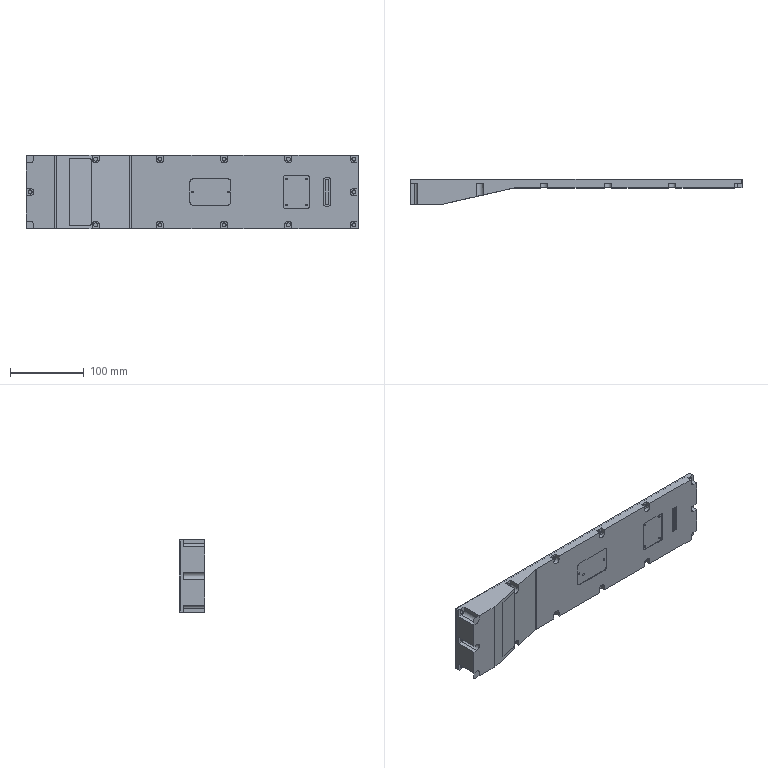CAM job | Mastercam | 3-axis milling, 5-axis milling, drilling | part box 450 x 35 x 100 mm | stock box 458 x 40 x 105 mm
Tools:
tool_number,name,type,diameter_mm,corner_radius_mm,flutes,flute_length_mm,overall_length_mm,shoulder_length_mm,holder_diameter_mm,length_offset,diameter_offset,default_rpm,default_feed_mm_min,default_plunge_mm_min,coolant
1,4 Ball Mill / Bull Nose Mill,ball end mill,4,2,4,25,100,30,50,1,1,7000,1000,600,COOL_OFF
2,3 Flat End Mill,end mill,3,0,4,25,75,25,50,2,2,7000,1000,600,COOL_OFF
4,4 Flat End Mill,end mill,4,0,4,25,75,25,50,4,4,7000,3000,600,COOL_OFF
5,6 Flat End Mill,end mill,6,0,4,25,75,25,50,5,5,5000,2000,600,COOL_OFF
6,6 Flat End Mill,end mill,6,0,4,25,75,25,50,6,6,7000,3000,600,COOL_OFF
7,6 Chamfer Mill,chamfer mill,6,0,4,25,75,30,50,7,7,7000,1000,600,COOL_OFF
8,8 Flat End Mill,end mill,8,0,4,25,75,25,50,8,8,7000,3000,600,COOL_OFF
11,10 Bull Nose Mill,bull end mill,10,1,4,25,100,25,50,11,11,8000,4500,600,COOL_OFF
12,12 Flat End Mill,end mill,12,0,4,25,75,25,50,12,12,7000,4000,600,COOL_OFF
13,12 Flat End Mill,end mill,12,0,4,25,75,25,50,13,13,7000,1000,600,COOL_OFF
20,20 Flat End Mill,end mill,20,0,4,25,75,25,50,20,20,4000,4000,600,COOL_OFF
24,100 Flat End Mill,end mill,100,0,4,25,75,25,50,24,24,4000,1000,600,COOL_OFF
24,63 Flat End Mill,end mill,63,0,4,63,126,75.6,50,24,24,4000,1000,600,COOL_FLOOD
24,100 Flat End Mill,end mill,100,0,4,100,200,120,50,24,24,7000,4000,600,COOL_OFF
Operations:
seq,operation,operation_type,tool_number,tool_name,tool_diameter_mm,spindle_rpm,feed_mm_min,plunge_mm_min,retract_mm_min,cycle_time_s,wcs,posted,nc_file
1,Facing - [WCS: Plane] - [Tplane: Plane],Facing,24,100 Flat End Mill,100,4000,1000,600,1200,79.071,Plane,yes,.nc
2,2D High Speed (2D Dynamic Mill) - [WCS: Plane] - [Tplane: Plane],HighSpeed2D,12,12 Flat End Mill,12,7000,4000,600,1200,213.669,Plane,yes,.nc
3,3D High Speed (Area rest roughing) - [WCS: Plane] - [Tplane: Plane],HighSpeed3D,20,20 Flat End Mill,20,7000,4000,600,1200,1289.872,Plane,yes,.nc
4,Contour (2D chamfer) - [WCS: Plane] - [Tplane: Plane],Contour,7,6 Chamfer Mill,6,7000,1000,600,1200,12.114,Plane,yes,.nc
5,Contour (2D chamfer) - [WCS: Plane] - [Tplane: Plane],Contour,7,6 Chamfer Mill,6,7000,1000,600,1200,44.106,Plane,yes,.nc
6,Manual Entry (M00),ManualEntry,,,,0,0,0,0,0,Plane,yes,.nc
7,Facing - [WCS: Plane] - [Tplane: Plane],Facing,24,100 Flat End Mill,100,4000,1000,600,1200,79.071,Plane,yes,.nc
8,Contour (2D) - [WCS: Plane] - [Tplane: Plane],Contour,12,12 Flat End Mill,12,7000,1000,600,1200,428.756,Plane,yes,.nc
9,Stock model - [WCS: Plane] - [Tplane: Plane] - 1,139,,,,0,0,0,0,0,Plane,yes,.nc
10,Facing - [WCS: Plane-1] - [Tplane: Plane-1],Facing,24,100 Flat End Mill,100,4000,3000,600,1200,240.099,Plane-1,yes,.nc
11,3D High Speed (Area roughing) - [WCS: Plane-1] - [Tplane: Plane-1],HighSpeed3D,12,12 Flat End Mill,12,7000,4000,600,1200,1481.773,Plane-1,yes,.nc
12,Contour (2D chamfer) - [WCS: Plane-1] - [Tplane: Plane-1],Contour,7,6 Chamfer Mill,6,7000,1000,600,1200,66.938,Plane-1,yes,.nc
13,Manual Entry (松),ManualEntry,,,,0,0,0,0,0,Plane-1,yes,.nc
14,Manual Entry (M00),ManualEntry,,,,0,0,0,0,0,Plane-1,yes,.nc
15,Facing - [WCS: Plane-1] - [Tplane: Plane-1],Facing,24,100 Flat End Mill,100,4000,1000,600,1200,79.371,Plane-1,yes,.nc
16,Stock model - [WCS: Plane] - [Tplane: Plane-1] - 2,139,,,,0,0,0,0,0,Plane,yes,.nc
17,Facing - [WCS: Plane] - [Tplane: Plane],Facing,24,100 Flat End Mill,100,4000,1000,600,1200,79.071,Plane,no,
18,2D High Speed (2D Dynamic Mill) - [WCS: Plane] - [Tplane: Plane],HighSpeed2D,12,12 Flat End Mill,12,7000,4000,600,1200,133.12,Plane,no,
19,3D High Speed (Area rest roughing) - [WCS: Plane] - [Tplane: Plane],HighSpeed3D,20,20 Flat End Mill,20,7000,4000,600,1200,1149.39,Plane,no,
20,Contour (2D) - [WCS: Plane] - [Tplane: Plane],Contour,12,12 Flat End Mill,12,7000,1000,600,1200,428.723,Plane,no,
21,Contour (2D chamfer) - [WCS: Plane] - [Tplane: Plane],Contour,7,6 Chamfer Mill,6,7000,1000,600,1200,12.114,Plane,no,
22,Contour (2D chamfer) - [WCS: Plane] - [Tplane: Plane],Contour,7,6 Chamfer Mill,6,7000,1000,600,1200,44.106,Plane,no,
23,Manual Entry (松),ManualEntry,,,,0,0,0,0,0,Plane,no,
24,Facing - [WCS: Plane] - [Tplane: Plane],Facing,24,100 Flat End Mill,100,4000,1000,600,1200,79.071,Plane,no,
25,Manual Entry (加 1.5),ManualEntry,,,,0,0,0,0,0,Plane,yes,.nc
26,Facing - [WCS: Plane] - [Tplane: Plane],Facing,24,100 Flat End Mill,100,4000,1000,600,1200,79.071,Plane,yes,.nc
27,3D High Speed (Area rest roughing) - [WCS: Plane] - [Tplane: Plane],HighSpeed3D,12,12 Flat End Mill,12,8000,4000,600,1200,630.05,Plane,yes,.nc
28,Contour (Ramp) - [WCS: Plane] - [Tplane: Plane],Contour,8,8 Flat End Mill,8,7000,3000,600,1200,79.853,Plane,yes,.nc
29,Contour (Ramp) - [WCS: Plane] - [Tplane: Plane],Contour,8,8 Flat End Mill,8,7000,3000,600,1200,20.062,Plane,yes,.nc
30,Contour (Ramp) - [WCS: Plane] - [Tplane: Plane],Contour,8,8 Flat End Mill,8,7000,3000,600,1200,41.435,Plane,yes,.nc
31,Contour (2D) - [WCS: Plane] - [Tplane: Plane],Contour,8,8 Flat End Mill,8,7000,1000,600,1200,20.617,Plane,yes,.nc
32,Contour (2D) - [WCS: Plane] - [Tplane: Plane],Contour,8,8 Flat End Mill,8,7000,1000,600,1200,12.265,Plane,yes,.nc
33,Contour (2D) - [WCS: Plane] - [Tplane: Plane],Contour,8,8 Flat End Mill,8,7000,3000,600,1200,73.881,Plane,yes,.nc
34,Contour (2D) - [WCS: Plane] - [Tplane: Plane],Contour,8,8 Flat End Mill,8,7000,1000,600,1200,44.7,Plane,yes,.nc
35,Contour (2D) - [WCS: Plane] - [Tplane: Plane],Contour,8,8 Flat End Mill,8,7000,1000,600,1200,3.891,Plane,yes,.nc
36,2D High Speed (2D Area Mill) - [WCS: Plane] - [Tplane: Plane],HighSpeed2D,8,8 Flat End Mill,8,7000,3000,600,1200,28.618,Plane,yes,.nc
37,Contour (Ramp) - [WCS: Plane] - [Tplane: Plane],Contour,6,6 Flat End Mill,6,6000,2500,600,1200,11.519,Plane,yes,.nc
38,Contour (Remachining) - [WCS: Plane] - [Tplane: Plane],Contour,4,4 Flat End Mill,4,6000,2500,600,1200,10.678,Plane,yes,.nc
39,2D High Speed (2D Area Mill) - [WCS: Plane] - [Tplane: Plane],HighSpeed2D,4,4 Flat End Mill,4,6000,1000,600,1200,94.989,Plane,yes,.nc
40,Contour (2D) - [WCS: Plane] - [Tplane: Plane],Contour,4,4 Flat End Mill,4,6000,1000,600,1200,20.207,Plane,yes,.nc
41,Contour (Ramp) - [WCS: Plane] - [Tplane: Plane],Contour,4,4 Flat End Mill,4,6000,3000,600,1200,11.231,Plane,yes,.nc
42,Contour (Remachining) - [WCS: Plane] - [Tplane: Plane],Contour,4,4 Flat End Mill,4,6000,3000,600,1200,3.594,Plane,yes,.nc
43,Contour (Remachining) - [WCS: Plane] - [Tplane: Plane],Contour,4,4 Flat End Mill,4,6000,3000,600,1200,2.812,Plane,yes,.nc
44,Contour (Ramp) - [WCS: Plane] - [Tplane: Plane],Contour,4,4 Flat End Mill,4,6000,1000,600,1200,5.65,Plane,yes,.nc
45,Contour (2D) - [WCS: Plane] - [Tplane: Plane],Contour,4,4 Flat End Mill,4,6000,500,600,1200,8.517,Plane,yes,.nc
46,Surface Finish Flowline - [WCS: Plane] - [Tplane: Plane],MultiSurfaceFinishFlowline,11,10 Bull Nose Mill,10,8000,4500,600,1200,1039.438,Plane,yes,.nc
47,Contour (2D) - [WCS: Plane] - [Tplane: Plane],Contour,13,12 Flat End Mill,12,7000,1000,600,1200,274.108,Plane,yes,.nc
48,Facing - [WCS: Plane] - [Tplane: Plane],Facing,13,12 Flat End Mill,12,7000,1000,600,1200,37.511,Plane,yes,.nc
49,Contour (2D) - [WCS: Plane] - [Tplane: Plane],Contour,13,12 Flat End Mill,12,7000,1000,600,1200,287.632,Plane,yes,.nc
50,Drill/Counterbore - [WCS: Plane] - [Tplane: Plane],Drill,7,6 Chamfer Mill,6,3000,300,600,1200,17.119,Plane,yes,.nc
51,Deburr 5-axis - [WCS: Plane] - [Tplane: Plane],459,1,4 Ball Mill / Bull Nose Mill,4,7000,1000,600,1200,163.755,Plane,yes,.nc
52,3D High Speed (Area rest roughing) - [WCS: Plane-2] - [Tplane: Plane-2],HighSpeed3D,12,12 Flat End Mill,12,7000,4000,600,1200,908.264,Plane-2,yes,.nc
53,3D High Speed (Waterline rest passes) - [WCS: Plane-2] - [Tplane: Plane-2],HighSpeed3D,8,8 Flat End Mill,8,7000,3000,600,1200,213.021,Plane-2,yes,.nc
54,Contour (2D) - [WCS: Plane-2] - [Tplane: Plane-2],Contour,8,8 Flat End Mill,8,7000,1000,600,1200,67.548,Plane-2,yes,.nc
55,3D High Speed (Horizontal) - [WCS: Plane-2] - [Tplane: Plane-2],HighSpeed3D,8,8 Flat End Mill,8,7000,1000,600,1200,104.647,Plane-2,yes,.nc
56,3D High Speed (Horizontal) - [WCS: Plane-2] - [Tplane: Plane-2],HighSpeed3D,8,8 Flat End Mill,8,7000,1000,600,1200,49.242,Plane-2,yes,.nc
57,2D High Speed (2D Area Mill) - [WCS: Plane-2] - [Tplane: Plane-2],HighSpeed2D,8,8 Flat End Mill,8,7000,1000,600,1200,431.894,Plane-2,yes,.nc
58,Contour (2D) - [WCS: Plane-2] - [Tplane: Plane-2],Contour,8,8 Flat End Mill,8,7000,1000,600,1200,185.636,Plane-2,yes,.nc
59,3D High Speed (Waterline) - [WCS: Plane-2] - [Tplane: Plane-2],HighSpeed3D,8,8 Flat End Mill,8,7000,1000,600,1200,209.975,Plane-2,yes,.nc
60,3D High Speed (Waterline) - [WCS: Plane-2] - [Tplane: Plane-2],HighSpeed3D,8,8 Flat End Mill,8,7000,1000,600,1200,209.975,Plane-2,yes,.nc
61,Surface Finish Flowline - [WCS: Plane-2] - [Tplane: Plane-2],MultiSurfaceFinishFlowline,8,8 Flat End Mill,8,7000,4000,600,1200,1241.314,Plane-2,yes,.nc
62,Helix Bore - [WCS: Plane-2] - [Tplane: Plane-2],HelixBore,2,3 Flat End Mill,3,7000,1000,600,1200,12.195,Plane-2,yes,.nc
63,Drill/Counterbore - [WCS: Plane-2] - [Tplane: Plane-2],Drill,7,6 Chamfer Mill,6,3000,300,600,1200,18.281,Plane-2,yes,.nc
64,Deburr 5-axis - [WCS: Plane-2] - [Tplane: Plane-2],459,1,4 Ball Mill / Bull Nose Mill,4,7000,1000,600,1200,267.346,Plane-2,yes,.nc
65,3D High Speed (Area roughing) - [WCS: Plane-3] - [Tplane: Plane-3],HighSpeed3D,8,8 Flat End Mill,8,7000,3000,600,1200,130.756,Plane-3,yes,.nc
66,3D High Speed (Waterline rest passes) - [WCS: Plane-3] - [Tplane: Plane-3],HighSpeed3D,4,4 Flat End Mill,4,7000,3000,600,1200,52.385,Plane-3,yes,.nc
67,Contour (2D) - [WCS: Plane-3] - [Tplane: Plane-3],Contour,4,4 Flat End Mill,4,7000,1000,600,1200,14.333,Plane-3,yes,.nc
68,Contour (2D) - [WCS: Plane-3] - [Tplane: Plane-3],Contour,4,4 Flat End Mill,4,7000,1000,600,1200,13.376,Plane-3,yes,.nc
69,Contour (2D chamfer) - [WCS: Plane-3] - [Tplane: Plane-3],Contour,7,6 Chamfer Mill,6,7000,1000,600,1200,28.469,Plane-3,yes,.nc
70,Facing - [WCS: Plane-2] - [Tplane: Plane-2],Facing,24,100 Flat End Mill,100,4000,3000,600,1200,240.109,Plane-2,no,
71,Contour (2D) - [WCS: Plane] - [Tplane: Plane],Contour,8,8 Flat End Mill,8,7000,1000,600,1200,207.224,Plane,no,
72,Contour (2D) - [WCS: Plane] - [Tplane: Plane],Contour,8,8 Flat End Mill,8,7000,1000,600,1200,18.346,Plane,no,
73,Contour (Remachining) - [WCS: Plane] - [Tplane: Plane],Contour,4,4 Flat End Mill,4,6000,2500,600,1200,10.678,Plane,no,
74,2D High Speed (2D Area Mill) - [WCS: Plane] - [Tplane: Plane],HighSpeed2D,4,4 Flat End Mill,4,6000,1000,600,1200,94.989,Plane,no,
75,Contour (2D) - [WCS: Plane] - [Tplane: Plane],Contour,4,4 Flat End Mill,4,6000,1000,600,1200,20.207,Plane,no,
76,2D High Speed (2D Area Mill) - [WCS: Plane-2] - [Tplane: Plane-2],HighSpeed2D,8,8 Flat End Mill,8,7000,1000,600,1200,431.894,Plane-2,yes,.nc
77,3D High Speed (Waterline) - [WCS: Plane-2] - [Tplane: Plane-2],HighSpeed3D,8,8 Flat End Mill,8,7000,1000,600,1200,232.854,Plane-2,yes,.nc
78,3D High Speed (Horizontal) - [WCS: Plane-2] - [Tplane: Plane-2],HighSpeed3D,8,8 Flat End Mill,8,7000,1000,600,1200,49.242,Plane-2,yes,.nc
79,Surface Finish Flowline - [WCS: Plane-2] - [Tplane: Plane-2],MultiSurfaceFinishFlowline,8,8 Flat End Mill,8,7000,4000,600,1200,1241.314,Plane-2,yes,.nc